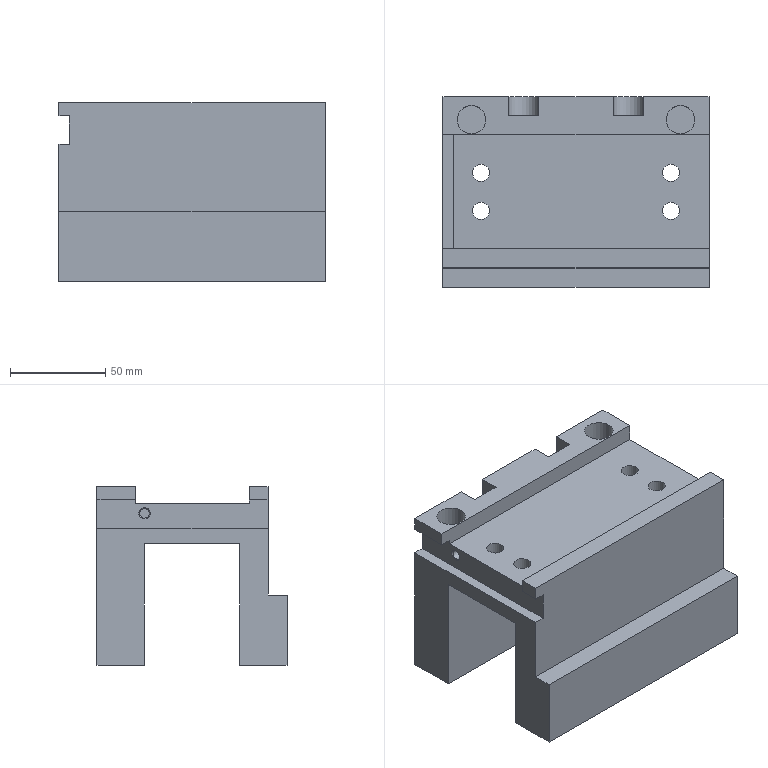Part | STEP file | Tube feed_id918_x_t | 1 solid | 67 faces | box 140 x 100 x 94 mm | volume 657707 mm3 | plane 35 | cylinder 19 | cone 13 | commonest cylinder face diameters 8.5 x6 9 x4 10 x4 15 x2 16 x2 5 x1